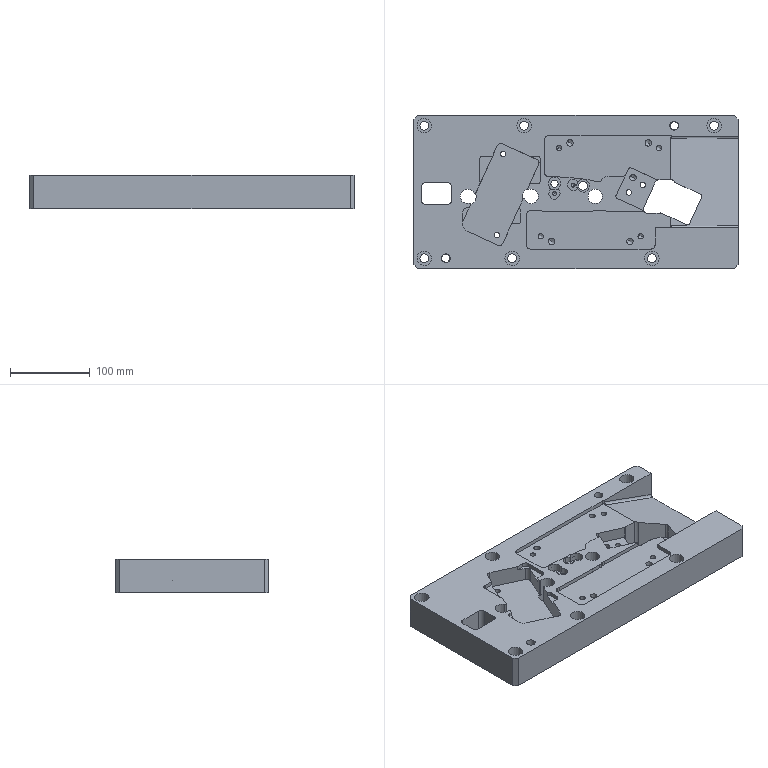Part | CATIA | 1 solid | 233 faces | box 406 x 192 x 42 mm | volume 2564090 mm3 | cylinder 133 | plane 72 | cone 26 | other 2 | commonest cylinder face diameters 10 x32 11 x18 18 x18 6.8 x16 8 x10 6 x8